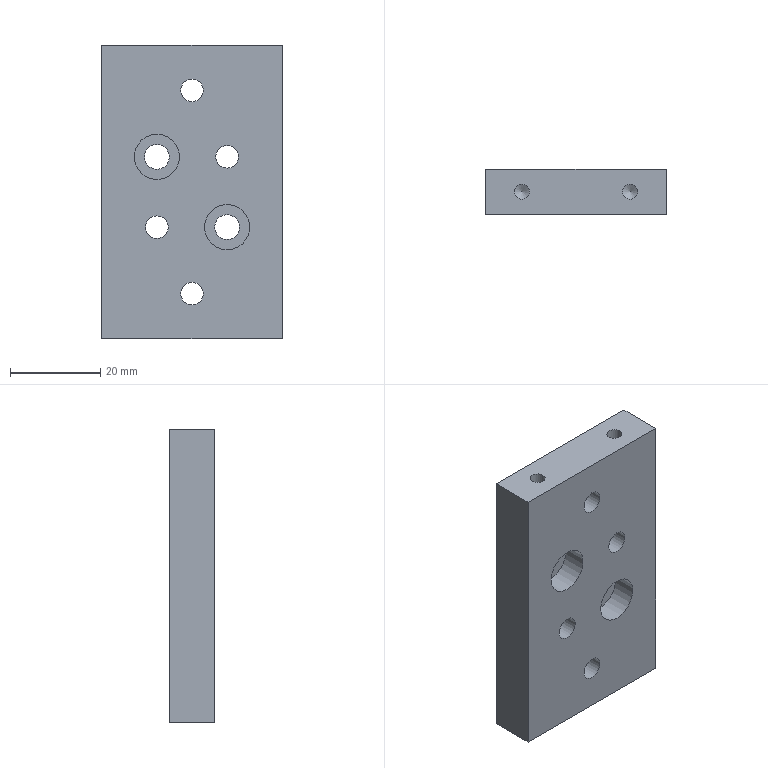Part | NX | features BREP 1 | 1 solid | 20 faces | box 40 x 10 x 65 mm | volume 23969 mm3 | cylinder 10 | plane 8 | cone 2 | commonest cylinder face diameters 5 x4 3.3 x2 5.5 x2 10 x2
STEP:
#1=CARTESIAN_POINT('',(20.,-5.,32.5));
#2=VERTEX_POINT('',#1);
#3=CARTESIAN_POINT('',(20.,-5.,-32.5));
#4=VERTEX_POINT('',#3);
#5=CARTESIAN_POINT('',(20.,-5.,32.5));
#6=DIRECTION('',(0.,0.,-1.));
#7=VECTOR('',#6,1000.);
#8=LINE('',#5,#7);
#9=EDGE_CURVE('',#2,#4,#8,.T.);
#10=ORIENTED_EDGE('',*,*,#9,.T.);
#11=CARTESIAN_POINT('',(20.,5.,-32.5));
#12=VERTEX_POINT('',#11);
#13=CARTESIAN_POINT('',(20.,5.,-32.5));
#14=DIRECTION('',(0.,-1.,0.));
#15=VECTOR('',#14,1000.);
#16=LINE('',#13,#15);
#17=EDGE_CURVE('',#12,#4,#16,.T.);
#18=ORIENTED_EDGE('',*,*,#17,.F.);
#19=CARTESIAN_POINT('',(20.,5.,32.5));
#20=VERTEX_POINT('',#19);
#21=CARTESIAN_POINT('',(20.,5.,32.5));
#22=DIRECTION('',(0.,0.,-1.));
#23=VECTOR('',#22,1000.);
#24=LINE('',#21,#23);
#25=EDGE_CURVE('',#20,#12,#24,.T.);
#26=ORIENTED_EDGE('',*,*,#25,.F.);
#27=CARTESIAN_POINT('',(20.,5.,32.5));
#28=DIRECTION('',(0.,-1.,0.));
#29=VECTOR('',#28,1000.);
#30=LINE('',#27,#29);
#31=EDGE_CURVE('',#20,#2,#30,.T.);
#32=ORIENTED_EDGE('',*,*,#31,.T.);
#33=EDGE_LOOP('',(#10,#18,#26,#32));
#34=FACE_BOUND('',#33,.T.);
#35=CARTESIAN_POINT('',(20.,5.,32.5));
#36=DIRECTION('',(-1.,0.,0.));
#37=DIRECTION('',(0.,0.,-1.));
#38=AXIS2_PLACEMENT_3D('',#35,#36,#37);
#39=PLANE('',#38);
#40=ADVANCED_FACE('',(#34),#39,.F.);
#41=CARTESIAN_POINT('',(-20.,-5.,-32.5));
#42=VERTEX_POINT('',#41);
#43=CARTESIAN_POINT('',(-20.,-5.,-32.5));
#44=DIRECTION('',(-1.,0.,0.));
#45=VECTOR('',#44,1000.);
#46=LINE('',#43,#45);
#47=EDGE_CURVE('',#4,#42,#46,.T.);
#48=ORIENTED_EDGE('',*,*,#47,.T.);
#49=CARTESIAN_POINT('',(-20.,5.,-32.5));
#50=VERTEX_POINT('',#49);
#51=CARTESIAN_POINT('',(-20.,5.,-32.5));
#52=DIRECTION('',(0.,-1.,0.));
#53=VECTOR('',#52,1000.);
#54=LINE('',#51,#53);
#55=EDGE_CURVE('',#50,#42,#54,.T.);
#56=ORIENTED_EDGE('',*,*,#55,.F.);
#57=CARTESIAN_POINT('',(-20.,5.,-32.5));
#58=DIRECTION('',(-1.,0.,0.));
#59=VECTOR('',#58,1000.);
#60=LINE('',#57,#59);
#61=EDGE_CURVE('',#12,#50,#60,.T.);
#62=ORIENTED_EDGE('',*,*,#61,.F.);
#63=ORIENTED_EDGE('',*,*,#17,.T.);
#64=EDGE_LOOP('',(#48,#56,#62,#63));
#65=FACE_BOUND('',#64,.T.);
#66=CARTESIAN_POINT('',(-20.,5.,-32.5));
#67=DIRECTION('',(0.,0.,1.));
#68=DIRECTION('',(-1.,0.,0.));
#69=AXIS2_PLACEMENT_3D('',#66,#67,#68);
#70=PLANE('',#69);
#71=ADVANCED_FACE('',(#65),#70,.F.);
#72=CARTESIAN_POINT('',(-20.,-5.,32.5));
#73=VERTEX_POINT('',#72);
#74=CARTESIAN_POINT('',(-20.,-5.,32.5));
#75=DIRECTION('',(0.,0.,1.));
#76=VECTOR('',#75,1000.);
#77=LINE('',#74,#76);
#78=EDGE_CURVE('',#42,#73,#77,.T.);
#79=ORIENTED_EDGE('',*,*,#78,.T.);
#80=CARTESIAN_POINT('',(-20.,5.,32.5));
#81=VERTEX_POINT('',#80);
#82=CARTESIAN_POINT('',(-20.,5.,32.5));
#83=DIRECTION('',(0.,-1.,0.));
#84=VECTOR('',#83,1000.);
#85=LINE('',#82,#84);
#86=EDGE_CURVE('',#81,#73,#85,.T.);
#87=ORIENTED_EDGE('',*,*,#86,.F.);
#88=CARTESIAN_POINT('',(-20.,5.,32.5));
#89=DIRECTION('',(0.,0.,1.));
#90=VECTOR('',#89,1000.);
#91=LINE('',#88,#90);
#92=EDGE_CURVE('',#50,#81,#91,.T.);
#93=ORIENTED_EDGE('',*,*,#92,.F.);
#94=ORIENTED_EDGE('',*,*,#55,.T.);
#95=EDGE_LOOP('',(#79,#87,#93,#94));
#96=FACE_BOUND('',#95,.T.);
#97=CARTESIAN_POINT('',(-20.,5.,32.5));
#98=DIRECTION('',(1.,0.,0.));
#99=DIRECTION('',(0.,0.,1.));
#100=AXIS2_PLACEMENT_3D('',#97,#98,#99);
#101=PLANE('',#100);
#102=ADVANCED_FACE('',(#96),#101,.F.);
#103=CARTESIAN_POINT('',(13.65,0.,32.5));
#104=VERTEX_POINT('',#103);
#105=CARTESIAN_POINT('',(12.,0.,32.5));
#106=DIRECTION('',(0.,0.,1.));
#107=DIRECTION('',(1.,0.,0.));
#108=AXIS2_PLACEMENT_3D('',#105,#106,#107);
#109=CIRCLE('',#108,1.65);
#110=EDGE_CURVE('',#104,#104,#109,.T.);
#111=ORIENTED_EDGE('',*,*,#110,.F.);
#112=EDGE_LOOP('',(#111));
#113=FACE_BOUND('',#112,.T.);
#114=CARTESIAN_POINT('',(-10.35,0.,32.5));
#115=VERTEX_POINT('',#114);
#116=CARTESIAN_POINT('',(-12.,0.,32.5));
#117=DIRECTION('',(0.,0.,1.));
#118=DIRECTION('',(1.,0.,0.));
#119=AXIS2_PLACEMENT_3D('',#116,#117,#118);
#120=CIRCLE('',#119,1.65);
#121=EDGE_CURVE('',#115,#115,#120,.T.);
#122=ORIENTED_EDGE('',*,*,#121,.F.);
#123=EDGE_LOOP('',(#122));
#124=FACE_BOUND('',#123,.T.);
#125=CARTESIAN_POINT('',(-20.,-5.,32.5));
#126=DIRECTION('',(1.,0.,0.));
#127=VECTOR('',#126,1000.);
#128=LINE('',#125,#127);
#129=EDGE_CURVE('',#73,#2,#128,.T.);
#130=ORIENTED_EDGE('',*,*,#129,.T.);
#131=ORIENTED_EDGE('',*,*,#31,.F.);
#132=CARTESIAN_POINT('',(-20.,5.,32.5));
#133=DIRECTION('',(1.,0.,0.));
#134=VECTOR('',#133,1000.);
#135=LINE('',#132,#134);
#136=EDGE_CURVE('',#81,#20,#135,.T.);
#137=ORIENTED_EDGE('',*,*,#136,.F.);
#138=ORIENTED_EDGE('',*,*,#86,.T.);
#139=EDGE_LOOP('',(#130,#131,#137,#138));
#140=FACE_BOUND('',#139,.T.);
#141=CARTESIAN_POINT('',(-20.,5.,32.5));
#142=DIRECTION('',(0.,0.,-1.));
#143=DIRECTION('',(1.,0.,0.));
#144=AXIS2_PLACEMENT_3D('',#141,#142,#143);
#145=PLANE('',#144);
#146=ADVANCED_FACE('',(#113,#124,#140),#145,.F.);
#147=CARTESIAN_POINT('',(0.,5.,-25.));
#148=VERTEX_POINT('',#147);
#149=CARTESIAN_POINT('',(0.,5.,-22.5));
#150=DIRECTION('',(0.,-1.,0.));
#151=DIRECTION('',(0.,0.,-1.));
#152=AXIS2_PLACEMENT_3D('',#149,#150,#151);
#153=CIRCLE('',#152,2.5);
#154=EDGE_CURVE('',#148,#148,#153,.T.);
#155=ORIENTED_EDGE('',*,*,#154,.T.);
#156=EDGE_LOOP('',(#155));
#157=FACE_BOUND('',#156,.T.);
#158=CARTESIAN_POINT('',(0.,5.,20.));
#159=VERTEX_POINT('',#158);
#160=CARTESIAN_POINT('',(0.,5.,22.5));
#161=DIRECTION('',(0.,-1.,0.));
#162=DIRECTION('',(0.,0.,-1.));
#163=AXIS2_PLACEMENT_3D('',#160,#161,#162);
#164=CIRCLE('',#163,2.5);
#165=EDGE_CURVE('',#159,#159,#164,.T.);
#166=ORIENTED_EDGE('',*,*,#165,.T.);
#167=EDGE_LOOP('',(#166));
#168=FACE_BOUND('',#167,.T.);
#169=CARTESIAN_POINT('',(-7.778,5.,-10.278));
#170=VERTEX_POINT('',#169);
#171=CARTESIAN_POINT('',(-7.778,5.,-7.778));
#172=DIRECTION('',(0.,-1.,0.));
#173=DIRECTION('',(0.,0.,-1.));
#174=AXIS2_PLACEMENT_3D('',#171,#172,#173);
#175=CIRCLE('',#174,2.5);
#176=EDGE_CURVE('',#170,#170,#175,.T.);
#177=ORIENTED_EDGE('',*,*,#176,.T.);
#178=EDGE_LOOP('',(#177));
#179=FACE_BOUND('',#178,.T.);
#180=CARTESIAN_POINT('',(7.778,5.,5.278));
#181=VERTEX_POINT('',#180);
#182=CARTESIAN_POINT('',(7.778,5.,7.778));
#183=DIRECTION('',(0.,-1.,0.));
#184=DIRECTION('',(0.,0.,-1.));
#185=AXIS2_PLACEMENT_3D('',#182,#183,#184);
#186=CIRCLE('',#185,2.5);
#187=EDGE_CURVE('',#181,#181,#186,.T.);
#188=ORIENTED_EDGE('',*,*,#187,.T.);
#189=EDGE_LOOP('',(#188));
#190=FACE_BOUND('',#189,.T.);
#191=CARTESIAN_POINT('',(7.778,5.,-10.528));
#192=VERTEX_POINT('',#191);
#193=CARTESIAN_POINT('',(7.778,5.,-7.778));
#194=DIRECTION('',(0.,-1.,0.));
#195=DIRECTION('',(0.,0.,-1.));
#196=AXIS2_PLACEMENT_3D('',#193,#194,#195);
#197=CIRCLE('',#196,2.75);
#198=EDGE_CURVE('',#192,#192,#197,.T.);
#199=ORIENTED_EDGE('',*,*,#198,.T.);
#200=EDGE_LOOP('',(#199));
#201=FACE_BOUND('',#200,.T.);
#202=CARTESIAN_POINT('',(-7.778,5.,5.028));
#203=VERTEX_POINT('',#202);
#204=CARTESIAN_POINT('',(-7.778,5.,7.778));
#205=DIRECTION('',(0.,-1.,0.));
#206=DIRECTION('',(0.,0.,-1.));
#207=AXIS2_PLACEMENT_3D('',#204,#205,#206);
#208=CIRCLE('',#207,2.75);
#209=EDGE_CURVE('',#203,#203,#208,.T.);
#210=ORIENTED_EDGE('',*,*,#209,.T.);
#211=EDGE_LOOP('',(#210));
#212=FACE_BOUND('',#211,.T.);
#213=ORIENTED_EDGE('',*,*,#25,.T.);
#214=ORIENTED_EDGE('',*,*,#61,.T.);
#215=ORIENTED_EDGE('',*,*,#92,.T.);
#216=ORIENTED_EDGE('',*,*,#136,.T.);
#217=EDGE_LOOP('',(#213,#214,#215,#216));
#218=FACE_BOUND('',#217,.T.);
#219=CARTESIAN_POINT('',(0.,5.,0.));
#220=DIRECTION('',(0.,-1.,0.));
#221=DIRECTION('',(0.,0.,1.));
#222=AXIS2_PLACEMENT_3D('',#219,#220,#221);
#223=PLANE('',#222);
#224=ADVANCED_FACE('',(#157,#168,#179,#190,#201,#212,#218),#223,.F.);
#225=CARTESIAN_POINT('',(0.,-5.,-25.));
#226=VERTEX_POINT('',#225);
#227=CARTESIAN_POINT('',(0.,-5.,-22.5));
#228=DIRECTION('',(0.,-1.,0.));
#229=DIRECTION('',(0.,0.,-1.));
#230=AXIS2_PLACEMENT_3D('',#227,#228,#229);
#231=CIRCLE('',#230,2.5);
#232=EDGE_CURVE('',#226,#226,#231,.T.);
#233=ORIENTED_EDGE('',*,*,#232,.F.);
#234=EDGE_LOOP('',(#233));
#235=FACE_BOUND('',#234,.T.);
#236=CARTESIAN_POINT('',(0.,-5.,20.));
#237=VERTEX_POINT('',#236);
#238=CARTESIAN_POINT('',(0.,-5.,22.5));
#239=DIRECTION('',(0.,-1.,0.));
#240=DIRECTION('',(0.,0.,-1.));
#241=AXIS2_PLACEMENT_3D('',#238,#239,#240);
#242=CIRCLE('',#241,2.5);
#243=EDGE_CURVE('',#237,#237,#242,.T.);
#244=ORIENTED_EDGE('',*,*,#243,.F.);
#245=EDGE_LOOP('',(#244));
#246=FACE_BOUND('',#245,.T.);
#247=CARTESIAN_POINT('',(-7.778,-5.,-10.278));
#248=VERTEX_POINT('',#247);
#249=CARTESIAN_POINT('',(-7.778,-5.,-7.778));
#250=DIRECTION('',(0.,-1.,0.));
#251=DIRECTION('',(0.,0.,-1.));
#252=AXIS2_PLACEMENT_3D('',#249,#250,#251);
#253=CIRCLE('',#252,2.5);
#254=EDGE_CURVE('',#248,#248,#253,.T.);
#255=ORIENTED_EDGE('',*,*,#254,.F.);
#256=EDGE_LOOP('',(#255));
#257=FACE_BOUND('',#256,.T.);
#258=CARTESIAN_POINT('',(7.778,-5.,5.278));
#259=VERTEX_POINT('',#258);
#260=CARTESIAN_POINT('',(7.778,-5.,7.778));
#261=DIRECTION('',(0.,-1.,0.));
#262=DIRECTION('',(0.,0.,-1.));
#263=AXIS2_PLACEMENT_3D('',#260,#261,#262);
#264=CIRCLE('',#263,2.5);
#265=EDGE_CURVE('',#259,#259,#264,.T.);
#266=ORIENTED_EDGE('',*,*,#265,.F.);
#267=EDGE_LOOP('',(#266));
#268=FACE_BOUND('',#267,.T.);
#269=CARTESIAN_POINT('',(7.778,-5.,-12.778));
#270=VERTEX_POINT('',#269);
#271=CARTESIAN_POINT('',(7.778,-5.,-7.778));
#272=DIRECTION('',(0.,-1.,0.));
#273=DIRECTION('',(0.,0.,-1.));
#274=AXIS2_PLACEMENT_3D('',#271,#272,#273);
#275=CIRCLE('',#274,5.);
#276=EDGE_CURVE('',#270,#270,#275,.T.);
#277=ORIENTED_EDGE('',*,*,#276,.F.);
#278=EDGE_LOOP('',(#277));
#279=FACE_BOUND('',#278,.T.);
#280=CARTESIAN_POINT('',(-7.778,-5.,2.778));
#281=VERTEX_POINT('',#280);
#282=CARTESIAN_POINT('',(-7.778,-5.,7.778));
#283=DIRECTION('',(0.,-1.,0.));
#284=DIRECTION('',(0.,0.,-1.));
#285=AXIS2_PLACEMENT_3D('',#282,#283,#284);
#286=CIRCLE('',#285,5.);
#287=EDGE_CURVE('',#281,#281,#286,.T.);
#288=ORIENTED_EDGE('',*,*,#287,.F.);
#289=EDGE_LOOP('',(#288));
#290=FACE_BOUND('',#289,.T.);
#291=ORIENTED_EDGE('',*,*,#9,.F.);
#292=ORIENTED_EDGE('',*,*,#129,.F.);
#293=ORIENTED_EDGE('',*,*,#78,.F.);
#294=ORIENTED_EDGE('',*,*,#47,.F.);
#295=EDGE_LOOP('',(#291,#292,#293,#294));
#296=FACE_BOUND('',#295,.T.);
#297=CARTESIAN_POINT('',(0.,-5.,0.));
#298=DIRECTION('',(0.,-1.,0.));
#299=DIRECTION('',(0.,0.,1.));
#300=AXIS2_PLACEMENT_3D('',#297,#298,#299);
#301=PLANE('',#300);
#302=ADVANCED_FACE('',(#235,#246,#257,#268,#279,#290,#296),#301,.T.);
#303=ORIENTED_EDGE('',*,*,#209,.F.);
#304=EDGE_LOOP('',(#303));
#305=FACE_BOUND('',#304,.T.);
#306=CARTESIAN_POINT('',(-7.778,0.4,5.028));
#307=VERTEX_POINT('',#306);
#308=CARTESIAN_POINT('',(-7.778,0.4,7.778));
#309=DIRECTION('',(0.,-1.,0.));
#310=DIRECTION('',(0.,0.,-1.));
#311=AXIS2_PLACEMENT_3D('',#308,#309,#310);
#312=CIRCLE('',#311,2.75);
#313=EDGE_CURVE('',#307,#307,#312,.T.);
#314=ORIENTED_EDGE('',*,*,#313,.T.);
#315=EDGE_LOOP('',(#314));
#316=FACE_BOUND('',#315,.T.);
#317=CARTESIAN_POINT('',(-7.778,-5.,7.778));
#318=DIRECTION('',(0.,-1.,0.));
#319=DIRECTION('',(0.,0.,1.));
#320=AXIS2_PLACEMENT_3D('',#317,#318,#319);
#321=CYLINDRICAL_SURFACE('',#320,2.75);
#322=ADVANCED_FACE('',(#305,#316),#321,.F.);
#323=ORIENTED_EDGE('',*,*,#313,.F.);
#324=EDGE_LOOP('',(#323));
#325=FACE_BOUND('',#324,.T.);
#326=CARTESIAN_POINT('',(-7.778,0.4,2.778));
#327=VERTEX_POINT('',#326);
#328=CARTESIAN_POINT('',(-7.778,0.4,7.778));
#329=DIRECTION('',(0.,-1.,0.));
#330=DIRECTION('',(0.,0.,-1.));
#331=AXIS2_PLACEMENT_3D('',#328,#329,#330);
#332=CIRCLE('',#331,5.);
#333=EDGE_CURVE('',#327,#327,#332,.T.);
#334=ORIENTED_EDGE('',*,*,#333,.T.);
#335=EDGE_LOOP('',(#334));
#336=FACE_BOUND('',#335,.T.);
#337=CARTESIAN_POINT('',(-5.028,0.4,7.778));
#338=DIRECTION('',(0.,1.,0.));
#339=DIRECTION('',(0.,0.,-1.));
#340=AXIS2_PLACEMENT_3D('',#337,#338,#339);
#341=PLANE('',#340);
#342=ADVANCED_FACE('',(#325,#336),#341,.F.);
#343=ORIENTED_EDGE('',*,*,#333,.F.);
#344=EDGE_LOOP('',(#343));
#345=FACE_BOUND('',#344,.T.);
#346=ORIENTED_EDGE('',*,*,#287,.T.);
#347=EDGE_LOOP('',(#346));
#348=FACE_BOUND('',#347,.T.);
#349=CARTESIAN_POINT('',(-7.778,-5.,7.778));
#350=DIRECTION('',(0.,-1.,0.));
#351=DIRECTION('',(0.,0.,1.));
#352=AXIS2_PLACEMENT_3D('',#349,#350,#351);
#353=CYLINDRICAL_SURFACE('',#352,5.);
#354=ADVANCED_FACE('',(#345,#348),#353,.F.);
#355=ORIENTED_EDGE('',*,*,#198,.F.);
#356=EDGE_LOOP('',(#355));
#357=FACE_BOUND('',#356,.T.);
#358=CARTESIAN_POINT('',(7.778,0.4,-10.528));
#359=VERTEX_POINT('',#358);
#360=CARTESIAN_POINT('',(7.778,0.4,-7.778));
#361=DIRECTION('',(0.,-1.,0.));
#362=DIRECTION('',(0.,0.,-1.));
#363=AXIS2_PLACEMENT_3D('',#360,#361,#362);
#364=CIRCLE('',#363,2.75);
#365=EDGE_CURVE('',#359,#359,#364,.T.);
#366=ORIENTED_EDGE('',*,*,#365,.T.);
#367=EDGE_LOOP('',(#366));
#368=FACE_BOUND('',#367,.T.);
#369=CARTESIAN_POINT('',(7.778,-5.,-7.778));
#370=DIRECTION('',(0.,-1.,0.));
#371=DIRECTION('',(0.,0.,1.));
#372=AXIS2_PLACEMENT_3D('',#369,#370,#371);
#373=CYLINDRICAL_SURFACE('',#372,2.75);
#374=ADVANCED_FACE('',(#357,#368),#373,.F.);
#375=ORIENTED_EDGE('',*,*,#365,.F.);
#376=EDGE_LOOP('',(#375));
#377=FACE_BOUND('',#376,.T.);
#378=CARTESIAN_POINT('',(7.778,0.4,-12.778));
#379=VERTEX_POINT('',#378);
#380=CARTESIAN_POINT('',(7.778,0.4,-7.778));
#381=DIRECTION('',(0.,-1.,0.));
#382=DIRECTION('',(0.,0.,-1.));
#383=AXIS2_PLACEMENT_3D('',#380,#381,#382);
#384=CIRCLE('',#383,5.);
#385=EDGE_CURVE('',#379,#379,#384,.T.);
#386=ORIENTED_EDGE('',*,*,#385,.T.);
#387=EDGE_LOOP('',(#386));
#388=FACE_BOUND('',#387,.T.);
#389=CARTESIAN_POINT('',(10.528,0.4,-7.778));
#390=DIRECTION('',(0.,1.,0.));
#391=DIRECTION('',(0.,0.,-1.));
#392=AXIS2_PLACEMENT_3D('',#389,#390,#391);
#393=PLANE('',#392);
#394=ADVANCED_FACE('',(#377,#388),#393,.F.);
#395=ORIENTED_EDGE('',*,*,#385,.F.);
#396=EDGE_LOOP('',(#395));
#397=FACE_BOUND('',#396,.T.);
#398=ORIENTED_EDGE('',*,*,#276,.T.);
#399=EDGE_LOOP('',(#398));
#400=FACE_BOUND('',#399,.T.);
#401=CARTESIAN_POINT('',(7.778,-5.,-7.778));
#402=DIRECTION('',(0.,-1.,0.));
#403=DIRECTION('',(0.,0.,1.));
#404=AXIS2_PLACEMENT_3D('',#401,#402,#403);
#405=CYLINDRICAL_SURFACE('',#404,5.);
#406=ADVANCED_FACE('',(#397,#400),#405,.F.);
#407=ORIENTED_EDGE('',*,*,#187,.F.);
#408=EDGE_LOOP('',(#407));
#409=FACE_BOUND('',#408,.T.);
#410=ORIENTED_EDGE('',*,*,#265,.T.);
#411=EDGE_LOOP('',(#410));
#412=FACE_BOUND('',#411,.T.);
#413=CARTESIAN_POINT('',(7.778,-5.,7.778));
#414=DIRECTION('',(0.,-1.,0.));
#415=DIRECTION('',(0.,0.,1.));
#416=AXIS2_PLACEMENT_3D('',#413,#414,#415);
#417=CYLINDRICAL_SURFACE('',#416,2.5);
#418=ADVANCED_FACE('',(#409,#412),#417,.F.);
#419=ORIENTED_EDGE('',*,*,#176,.F.);
#420=EDGE_LOOP('',(#419));
#421=FACE_BOUND('',#420,.T.);
#422=ORIENTED_EDGE('',*,*,#254,.T.);
#423=EDGE_LOOP('',(#422));
#424=FACE_BOUND('',#423,.T.);
#425=CARTESIAN_POINT('',(-7.778,-5.,-7.778));
#426=DIRECTION('',(0.,-1.,0.));
#427=DIRECTION('',(0.,0.,1.));
#428=AXIS2_PLACEMENT_3D('',#425,#426,#427);
#429=CYLINDRICAL_SURFACE('',#428,2.5);
#430=ADVANCED_FACE('',(#421,#424),#429,.F.);
#431=ORIENTED_EDGE('',*,*,#165,.F.);
#432=EDGE_LOOP('',(#431));
#433=FACE_BOUND('',#432,.T.);
#434=ORIENTED_EDGE('',*,*,#243,.T.);
#435=EDGE_LOOP('',(#434));
#436=FACE_BOUND('',#435,.T.);
#437=CARTESIAN_POINT('',(0.,-5.,22.5));
#438=DIRECTION('',(0.,-1.,0.));
#439=DIRECTION('',(0.,0.,1.));
#440=AXIS2_PLACEMENT_3D('',#437,#438,#439);
#441=CYLINDRICAL_SURFACE('',#440,2.5);
#442=ADVANCED_FACE('',(#433,#436),#441,.F.);
#443=ORIENTED_EDGE('',*,*,#154,.F.);
#444=EDGE_LOOP('',(#443));
#445=FACE_BOUND('',#444,.T.);
#446=ORIENTED_EDGE('',*,*,#232,.T.);
#447=EDGE_LOOP('',(#446));
#448=FACE_BOUND('',#447,.T.);
#449=CARTESIAN_POINT('',(0.,-5.,-22.5));
#450=DIRECTION('',(0.,-1.,0.));
#451=DIRECTION('',(0.,0.,1.));
#452=AXIS2_PLACEMENT_3D('',#449,#450,#451);
#453=CYLINDRICAL_SURFACE('',#452,2.5);
#454=ADVANCED_FACE('',(#445,#448),#453,.F.);
#455=CARTESIAN_POINT('',(-12.,0.,21.409));
#456=VERTEX_POINT('',#455);
#457=VERTEX_LOOP('',#456);
#458=FACE_BOUND('',#457,.T.);
#459=CARTESIAN_POINT('',(-10.35,0.,22.4));
#460=VERTEX_POINT('',#459);
#461=CARTESIAN_POINT('',(-12.,0.,22.4));
#462=DIRECTION('',(0.,0.,1.));
#463=DIRECTION('',(1.,0.,0.));
#464=AXIS2_PLACEMENT_3D('',#461,#462,#463);
#465=CIRCLE('',#464,1.65);
#466=EDGE_CURVE('',#460,#460,#465,.T.);
#467=ORIENTED_EDGE('',*,*,#466,.T.);
#468=EDGE_LOOP('',(#467));
#469=FACE_BOUND('',#468,.T.);
#470=CARTESIAN_POINT('',(-12.,0.,22.4));
#471=DIRECTION('',(0.,0.,1.));
#472=DIRECTION('',(-1.,0.,0.));
#473=AXIS2_PLACEMENT_3D('',#470,#471,#472);
#474=CONICAL_SURFACE('',#473,1.65,1.03);
#475=ADVANCED_FACE('',(#458,#469),#474,.F.);
#476=ORIENTED_EDGE('',*,*,#466,.F.);
#477=EDGE_LOOP('',(#476));
#478=FACE_BOUND('',#477,.T.);
#479=ORIENTED_EDGE('',*,*,#121,.T.);
#480=EDGE_LOOP('',(#479));
#481=FACE_BOUND('',#480,.T.);
#482=CARTESIAN_POINT('',(-12.,0.,32.5));
#483=DIRECTION('',(0.,0.,1.));
#484=DIRECTION('',(-1.,0.,0.));
#485=AXIS2_PLACEMENT_3D('',#482,#483,#484);
#486=CYLINDRICAL_SURFACE('',#485,1.65);
#487=ADVANCED_FACE('',(#478,#481),#486,.F.);
#488=CARTESIAN_POINT('',(12.,0.,21.409));
#489=VERTEX_POINT('',#488);
#490=VERTEX_LOOP('',#489);
#491=FACE_BOUND('',#490,.T.);
#492=CARTESIAN_POINT('',(13.65,0.,22.4));
#493=VERTEX_POINT('',#492);
#494=CARTESIAN_POINT('',(12.,0.,22.4));
#495=DIRECTION('',(0.,0.,1.));
#496=DIRECTION('',(1.,0.,0.));
#497=AXIS2_PLACEMENT_3D('',#494,#495,#496);
#498=CIRCLE('',#497,1.65);
#499=EDGE_CURVE('',#493,#493,#498,.T.);
#500=ORIENTED_EDGE('',*,*,#499,.T.);
#501=EDGE_LOOP('',(#500));
#502=FACE_BOUND('',#501,.T.);
#503=CARTESIAN_POINT('',(12.,0.,22.4));
#504=DIRECTION('',(0.,0.,1.));
#505=DIRECTION('',(-1.,0.,0.));
#506=AXIS2_PLACEMENT_3D('',#503,#504,#505);
#507=CONICAL_SURFACE('',#506,1.65,1.03);
#508=ADVANCED_FACE('',(#491,#502),#507,.F.);
#509=ORIENTED_EDGE('',*,*,#499,.F.);
#510=EDGE_LOOP('',(#509));
#511=FACE_BOUND('',#510,.T.);
#512=ORIENTED_EDGE('',*,*,#110,.T.);
#513=EDGE_LOOP('',(#512));
#514=FACE_BOUND('',#513,.T.);
#515=CARTESIAN_POINT('',(12.,0.,32.5));
#516=DIRECTION('',(0.,0.,1.));
#517=DIRECTION('',(-1.,0.,0.));
#518=AXIS2_PLACEMENT_3D('',#515,#516,#517);
#519=CYLINDRICAL_SURFACE('',#518,1.65);
#520=ADVANCED_FACE('',(#511,#514),#519,.F.);
#521=CLOSED_SHELL('',(#40,#71,#102,#146,#224,#302,#322,#342,#354,#374,#394,#406,#418,#430,#442,#454,#475,#487,#508,#520));
#522=MANIFOLD_SOLID_BREP('',#521);
#523=(LENGTH_UNIT()NAMED_UNIT(*)SI_UNIT(.MILLI.,.METRE.));
#524=UNCERTAINTY_MEASURE_WITH_UNIT(LENGTH_MEASURE(0.00001),#523,'','');
#525=(NAMED_UNIT(*)PLANE_ANGLE_UNIT()SI_UNIT($,.RADIAN.));
#526=(NAMED_UNIT(*)SI_UNIT($,.STERADIAN.)SOLID_ANGLE_UNIT());
#527=(GEOMETRIC_REPRESENTATION_CONTEXT(3)GLOBAL_UNCERTAINTY_ASSIGNED_CONTEXT((#524))GLOBAL_UNIT_ASSIGNED_CONTEXT((#523,#525,#526))REPRESENTATION_CONTEXT('',''));
#528=ADVANCED_BREP_SHAPE_REPRESENTATION('',(#522),#527);